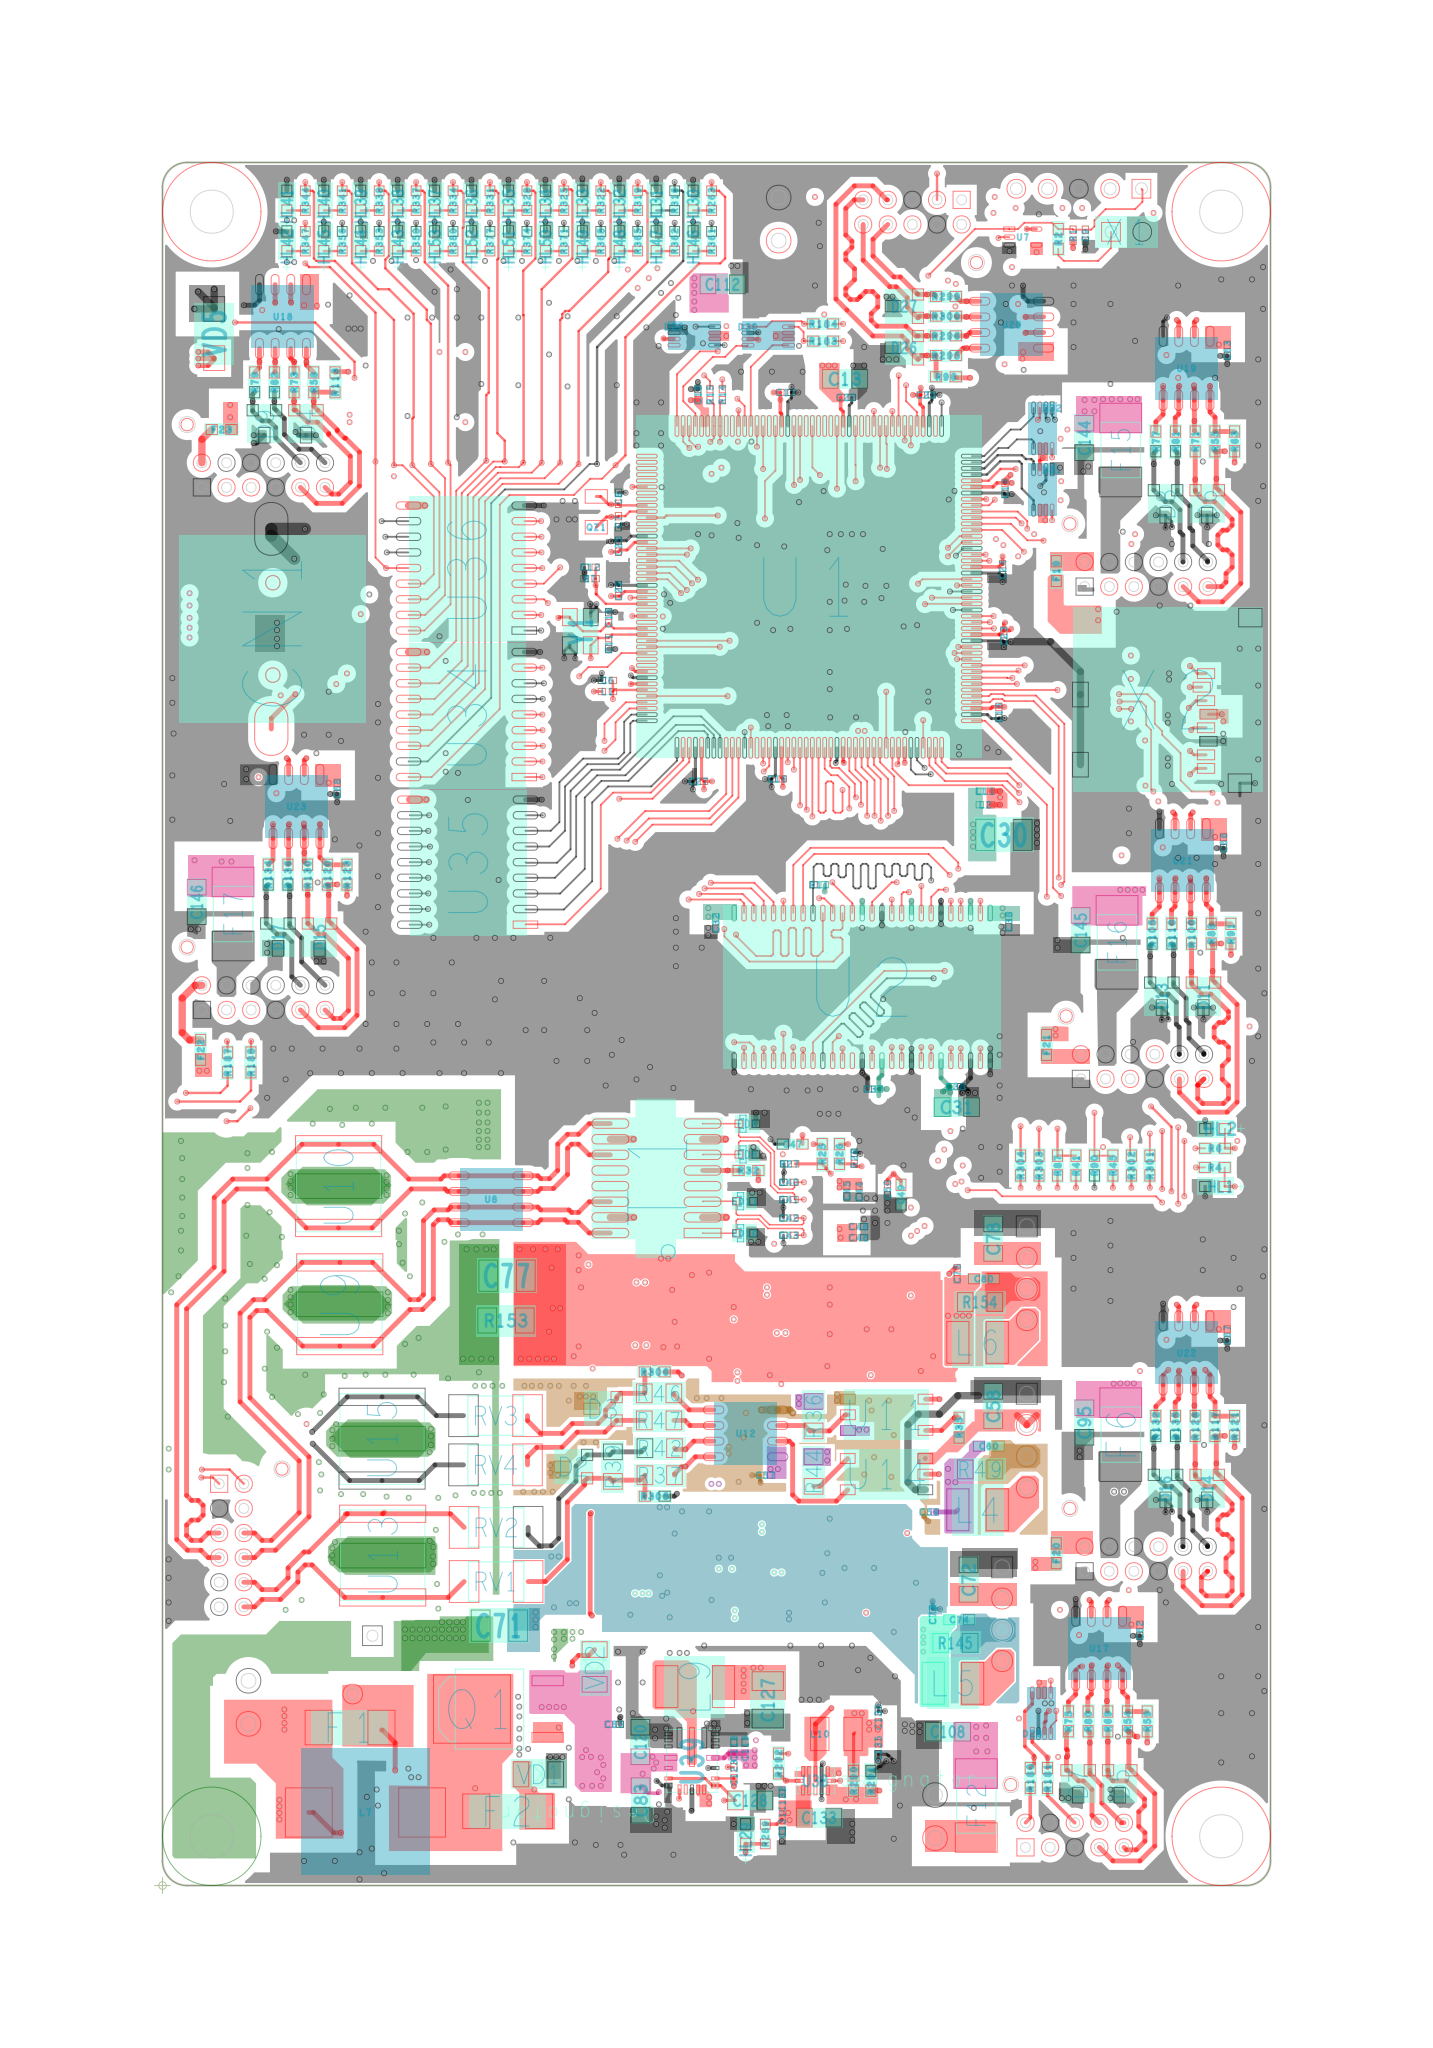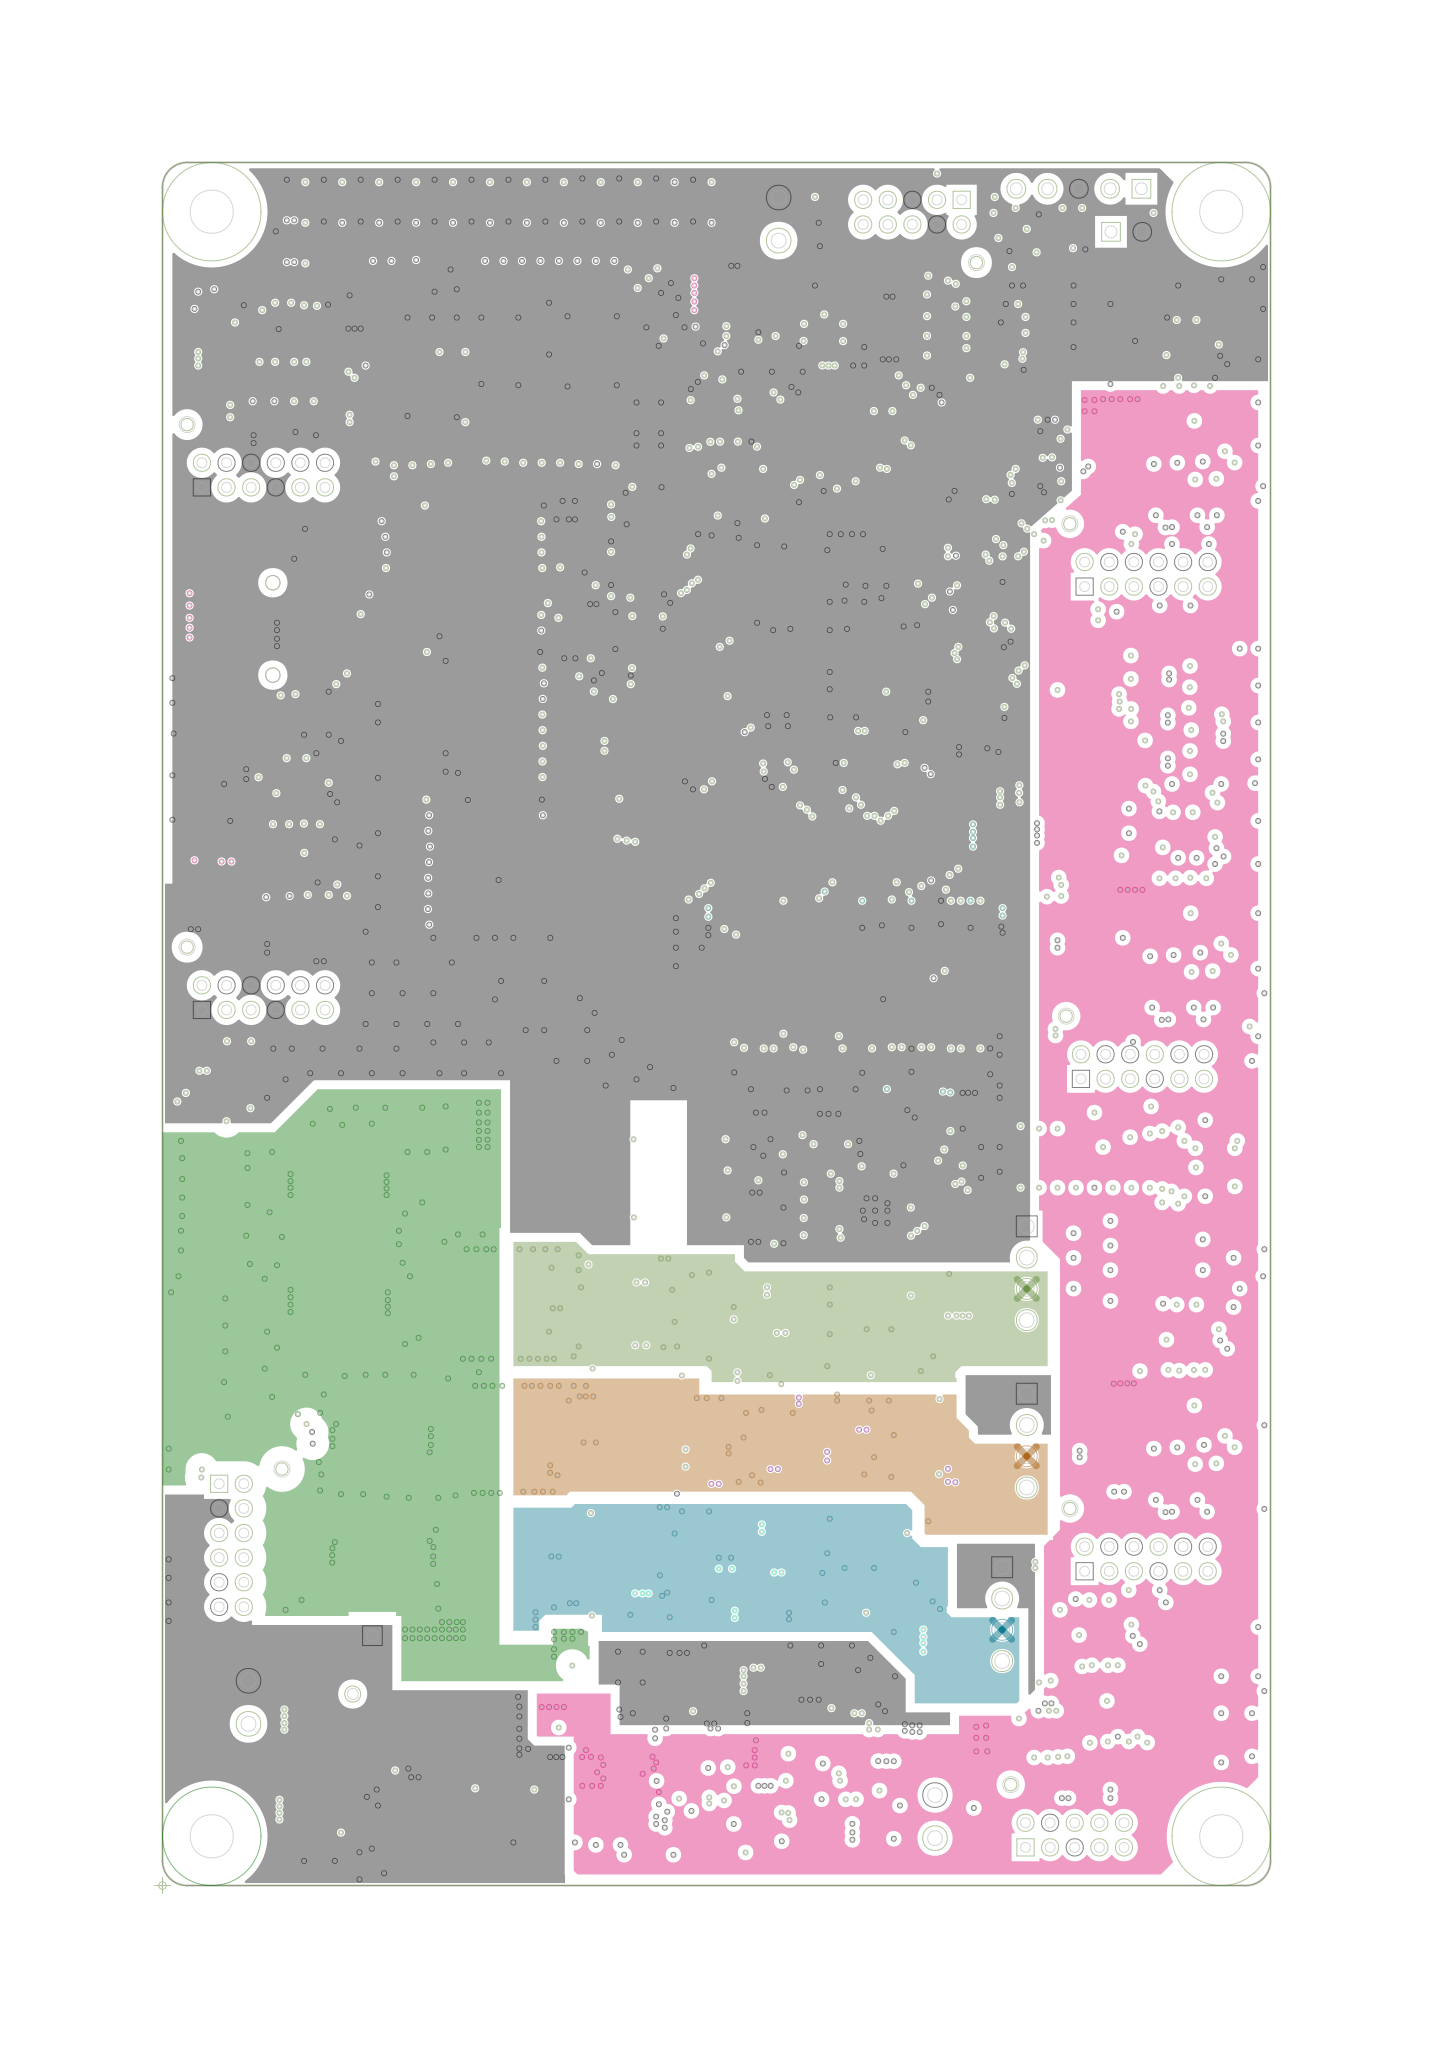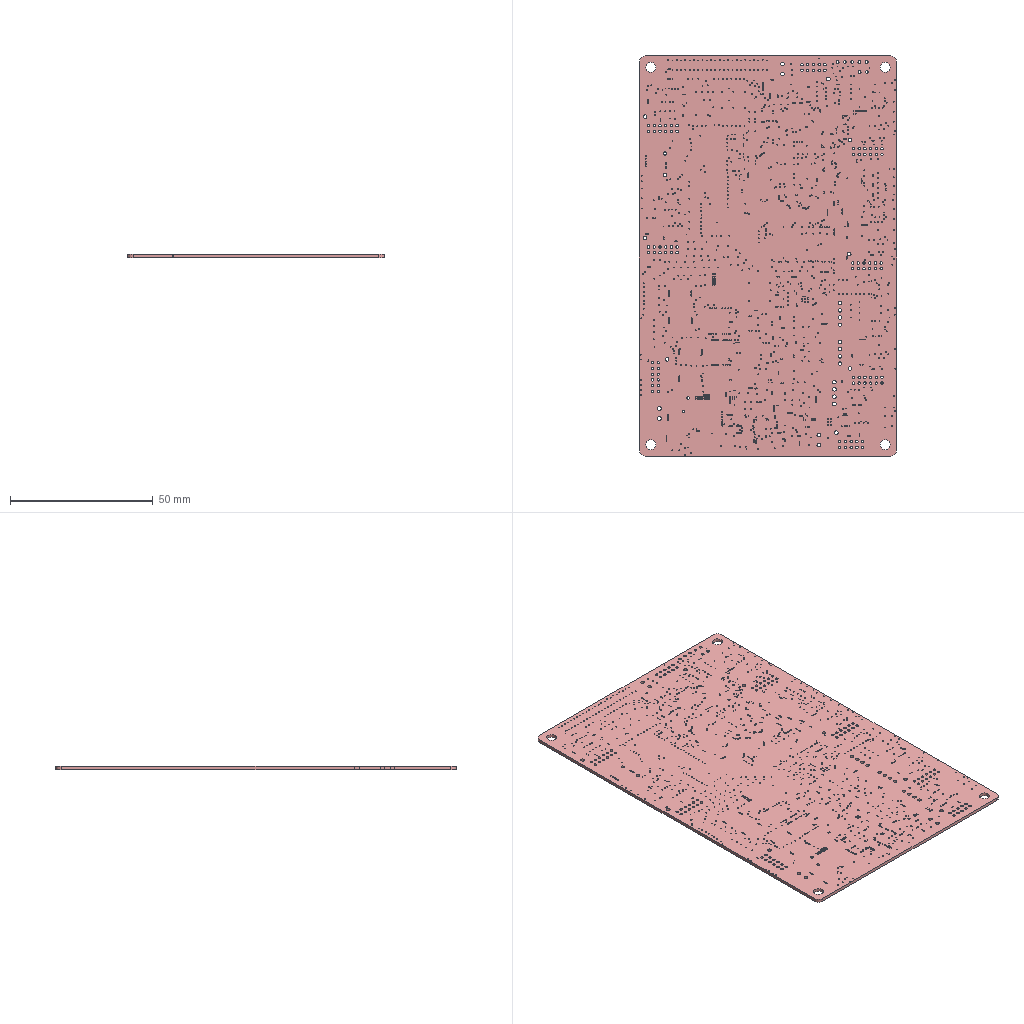Circuit board layout | Cadence Allegro | box 90 x 140 x 1.1 mm
Layer stack:
# Cadence Allegro layer stack of  (unit mm; from the constraint file cross-section; dielectric type: 0 not recorded (Allegro does not mark core vs prepreg), 3 surface material)
index,name,kind,layer,copper_thickness_mm,dielectric_type,dielectric_thickness_mm,dielectric_material,dielectric_constant
0,Top Surface,other,,,,,,
1,TOP,copper,TOP,0.0305,,,,
2,Dielectric1,dielectric,,,0,0.2032,FR-4,4.5
3,GND02,copper,GND02,0.0305,,,,
4,Dielectric2,dielectric,,,0,0.2032,FR-4,4.5
5,LAYER03,copper,LAYER03,0.0305,,,,
6,Dielectric3,dielectric,,,0,0.2032,FR-4,4.5
7,POWER04,copper,POWER04,0.0305,,,,
8,Dielectric4,dielectric,,,0,0.2032,FR-4,4.5
9,GND05,copper,GND05,0.0305,,,,
10,Dielectric5,dielectric,,,0,0.2032,FR-4,4.5
11,BOTTOM,copper,BOTTOM,0.0305,,,,
12,Bottom Surface,other,,,,,,
# drill layer pairs: low layer,high layer
drill_pair,TOP,BOTTOM
Part placement, first 524 of 796 lines:
REFDES,COMP_VALUE,SYM_NAME,SYM_X,SYM_Y,SYM_ROTATE,SYM_MIRROR
C1,2.2uf/16V,C0603,65.337,112.614,0.000,YES
C2,2.2uf/16V,C0603,59.537,92.914,270.000,YES
C3,1nf/50V,C0402,38.687,113.614,180.000,YES
C4,2.2uf/16V,C0603,37.237,97.914,270.000,YES
C5,0.1uf/50V,C0402,38.937,98.664,90.000,YES
C6,0.1uf/50V,C0402,36.587,97.914,180.000,NO
C7,6pf/50V,C0402,37.037,111.264,270.000,NO
C8,6pf/50V,C0402,37.037,112.264,90.000,NO
C9,0.1uf/50V,C0402,74.963,134.536,270.000,NO
C10,22pf/50V,C0402,36.237,102.564,90.000,NO
C11,22pf/50V,C0402,36.237,101.364,270.000,NO
C12,10nf/50V,C0402,35.187,107.114,180.000,NO
C13,4.7uf/50V,C0805,55.437,122.414,0.000,NO
C14,0.1uf/50V,C0402,55.487,90.514,0.000,YES
C15,0.1uf/50V,C0402,67.937,95.764,270.000,NO
C16,0.1uf/50V,C0402,50.387,89.914,180.000,NO
C17,0.1uf/50V,C0402,50.187,121.314,0.000,NO
C18,0.1uf/50V,C0402,43.486,120.687,90.000,NO
C19,0.1uf/50V,C0402,68.437,113.964,270.000,NO
C20,0.1uf/50V,C0402,60.737,91.964,270.000,YES
C21,4.7uf/50V,C0805,55.237,93.714,270.000,YES
C22,0.1uf/50V,C0402,55.087,120.914,0.000,NO
C23,0.1uf/50V,C0402,68.337,101.964,270.000,NO
C24,0.1uf/50V,C0402,68.237,107.364,270.000,NO
C25,0.1uf/50V,C0402,37.037,108.364,90.000,NO
C26,0.1uf/50V,C0402,37.037,104.764,90.000,NO
C27,0.1uf/50V,C0402,43.987,89.714,180.000,NO
C28,0.1uf/50V,C0402,61.587,121.114,0.000,NO
C29,10nf/50V,C0402,38.887,102.114,180.000,YES
C30,22uf/16V,C1210,68.349,85.363,0.000,NO
C31,4.7uf/50V,C0805,64.525,63.245,0.000,NO
C32,0.1uf/50V,C0402,44.937,78.664,270.000,NO
C33,0.1uf/50V,C0402,56.837,79.364,90.000,YES
C34,0.1uf/50V,C0402,60.837,79.364,90.000,YES
C35,0.1uf/50V,C0402,65.637,79.364,90.000,YES
C36,0.1uf/50V,C0402,68.737,78.764,270.000,NO
C37,0.1uf/50V,C0402,58.187,64.714,180.000,NO
C38,0.1uf/50V,C0402,63.987,64.914,0.000,NO
C39,0.1uf/50V,C0402,85.563,94.536,90.000,YES
C40,NC/10pF,C0402,51.336,57.137,180.000,NO
C41,NC/10pF,C0402,51.336,55.737,180.000,NO
C42,NC/10pF,C0402,51.336,54.237,180.000,NO
C43,NC/10pF,C0402,51.336,52.837,180.000,NO
C44,0.1uf/50V,C0402,56.586,56.837,270.000,NO
C45,0.1uf/50V,C0402,55.586,56.887,270.000,NO
C46,0.1uf/50V,C0402,56.086,52.637,0.000,NO
C47,10uf/16V,C0603,51.186,60.237,180.000,NO
C48,0.1uf/50V,C0402,56.086,53.537,0.000,NO
C49,10uf/16V,C0603,59.986,56.137,270.000,NO
C50,0.1uf/50V,C0402,58.886,56.987,270.000,NO
C51,0.1uf/50V,C0402,70.281,135.165,180.000,YES
C52,22pf/50V,C0402,58.136,59.037,0.000,YES
C53,22pf/50V,C0402,59.286,59.037,180.000,YES
C54,1NF/2KV,C1210,32.486,62.663,180.000,YES
C55,0.1uf/50V,C0402,44.936,60.663,0.000,YES
C56,0.1uf/50V,C0402,44.936,54.363,0.000,YES
C57,0.1uf/50V,C0402,49.436,33.337,180.000,NO
C58,4.7uf/50V,C0805,67.475,38.958,90.000,NO
C59,0.1uf/50V,C0402,62.736,30.352,180.000,NO
C60,10uf/16V,C0603,67.119,35.703,0.000,NO
C61,1NF/2KV,C1210,28.374,34.918,0.000,YES
C62,0.1uf/50V,C0402,79.386,21.187,270.000,NO
C63,0.1uf/50V,C0402,86.486,125.187,270.000,NO
C64,0.1uf/50V,C0402,12.550,129.200,180.000,YES
C65,0.1uf/50V,C0402,70.700,124.050,90.000,YES
C66,0.1uf/50V,C0402,86.186,85.187,270.000,NO
C67,0.1uf/50V,C0402,86.486,45.187,270.000,NO
C68,0.1uf/50V,C0402,14.186,89.587,270.000,NO
C69,0.1uf/50V,C0402,45.686,25.787,270.000,YES
C70,22pf/50V,C0402,34.186,21.887,270.000,YES
C71,1NF/2KV,C1210,27.363,21.114,180.000,NO
C72,4.7uf/50V,C0805,65.475,24.858,90.000,NO
C73,0.1uf/50V,C0402,62.552,21.564,90.000,NO
C74,10uf/16V,C0603,64.719,21.603,0.000,NO
C75,0.1uf/50V,C0402,64.552,49.264,90.000,NO
C76,22pf/50V,C0402,34.286,42.087,270.000,YES
C77,1NF/2KV,C1210,27.986,49.551,180.000,NO
C78,4.7uf/50V,C0805,67.475,52.558,90.000,NO
C79,0.1uf/50V,C0402,45.786,45.987,270.000,YES
C80,10uf/16V,C0603,66.719,49.303,0.000,NO
C83,10uf/50V,C0805,38.837,6.914,270.000,NO
C84,10uf/50V,C0805,38.763,6.614,90.000,YES
C85,0.1uf/50V,C0402,36.250,13.100,0.000,NO
C95,4.7uf/50V,C0805,74.879,37.619,270.000,NO
C96,0.1uf/50V,C0402,71.100,15.850,90.000,YES
C97,0.1uf/50V,C0402,71.850,12.500,0.000,YES
C102,0.1uf/50V,C0402,71.300,115.250,90.000,YES
C103,0.1uf/50V,C0402,71.300,111.650,270.000,YES
C105,0.1uf/50V,C0402,70.950,119.900,180.000,YES
C106,0.1uf/50V,C0402,71.300,116.650,270.000,YES
C108,4.7uf/50V,C0805,63.800,12.500,180.000,NO
C110,0.1uf/50V,C0402,45.050,125.900,0.000,YES
C111,0.1uf/50V,C0402,41.350,125.700,180.000,YES
C112,4.7uf/50V,C0805,45.500,130.100,0.000,NO
C113,0.1uf/50V,C0402,47.700,125.450,270.000,YES
C114,0.1uf/50V,C0402,50.450,125.900,180.000,YES
C115,10nf/50V,C0402,41.614,10.513,270.000,YES
C116,0.1uf/50V,C0402,40.714,10.513,270.000,YES
C117,0.1uf/50V,C0402,40.714,9.513,90.000,YES
C118,0.1uf/50V,C0402,46.414,10.713,90.000,NO
C119,10nf/50V,C0402,47.314,10.713,90.000,NO
C120,10uf/50V,C0805,38.814,11.663,90.000,NO
C121,10uf/50V,C0805,45.914,11.363,0.000,YES
C122,10uf/50V,C0805,38.714,11.263,270.000,YES
C123,0.47uf/25V,C0402,46.414,8.713,90.000,NO
C124,0.1uf/50V,C0402,43.850,6.600,0.000,YES
C125,22uf/16V,C1210,44.086,16.537,0.000,YES
C126,22uf/16V,C1210,49.137,15.086,90.000,YES
C127,22uf/16V,C1210,49.163,15.086,270.000,NO
C128,4.7uf/50V,C0805,47.737,6.914,0.000,NO
C129,0.1uf/50V,C0402,43.850,7.600,0.000,YES
C130,22uf/16V,C1210,53.437,4.814,180.000,YES
C131,10nf/50V,C0402,50.337,5.364,270.000,NO
C132,0.1uf/50V,C0402,50.337,6.564,90.000,NO
C133,10uf/50V,C0805,53.337,5.514,0.000,NO
C134,22pf/50V,C0402,56.137,7.764,270.000,YES
C135,0.1uf/50V,C0402,58.137,11.564,270.000,NO
C136,0.1uf/50V,C0402,58.137,13.264,90.000,NO
C137,22uf/16V,C1210,54.737,12.314,0.000,YES
C138,10nf/50V,C0402,54.350,8.500,0.000,YES
C139,0.1uf/50V,C0402,39.383,22.984,180.000,YES
C140,0.1uf/50V,C0402,39.483,43.184,180.000,YES
C141,1NF/2KV,C1210,33.586,17.437,270.000,YES
C142,10uf/50V,C0805,33.114,9.363,0.000,YES
C143,10uf/50V,C0805,35.763,12.686,270.000,YES
C144,4.7uf/50V,C0805,74.879,117.619,270.000,NO
C145,4.7uf/50V,C0805,74.579,77.619,270.000,NO
C146,4.7uf/50V,C0805,2.779,79.919,270.000,NO
C147,4.7uf/50V,C0805,6.981,101.021,180.000,YES
CN1,CR1220,CR1220,8.963,102.100,90.000,NO
D1,BAT54C,SOT23,13.163,99.472,0.000,YES
D2,SM712,SOT23,33.500,34.037,90.000,NO
D3,SM712,SOT23,35.900,38.737,90.000,NO
D4,SM712,SOT23,11.655,118.877,180.000,NO
D5,SM712,SOT23,77.755,8.377,180.000,NO
D6,SM712,SOT23,84.855,112.377,180.000,NO
D7,SM712,SOT23,74.376,8.377,180.000,NO
D8,SM712,SOT23,81.476,112.377,180.000,NO
D9,SM712,SOT23,8.276,118.877,180.000,NO
D11,SM712,SOT23,84.555,72.377,180.000,NO
D13,SM712,SOT23,81.176,72.377,180.000,NO
D14,SM712,SOT23,84.855,32.377,180.000,NO
D15,SM712,SOT23,12.755,77.177,180.000,NO
D16,SM712,SOT23,81.476,32.377,180.000,NO
D17,SM712,SOT23,9.376,77.177,180.000,NO
D18,SMC24,SOT23,33.100,25.937,90.000,YES
D19,TJA1044GT/3,SO8,43.926,28.142,0.000,YES
D20,SMC24,SOT23,33.000,46.137,90.000,YES
D21,TJA1044GT/3,SO8,44.026,48.342,0.000,YES
D26,SM712,SOT23,60.377,124.945,90.000,NO
D27,SM712,SOT23,60.377,128.324,90.000,NO
D28,TXS0102DCUR,VSSOP8,70.650,12.350,90.000,NO
D29,TXS0102DCUR,VSSOP8,41.551,126.659,0.000,NO
D30,TXS0102DCUR,VSSOP8,47.550,126.650,0.000,NO
D31,TXS0102DCUR,VSSOP8,72.259,115.049,270.000,NO
D32,TXS0102DCUR,VSSOP8,72.259,120.049,270.000,NO
ED8,ESD9X5VU,ESD5Z12T1,46.800,59.400,0.000,NO
ED9,ESD9X5VU,ESD5Z12T1,46.800,61.900,0.000,NO
ED10,ESD9X5VU,ESD5Z12T1,46.600,53.000,0.000,NO
ED11,ESD9X5VU,ESD5Z12T1,46.600,55.600,0.000,NO
F1,JFC2410-2100TS,JFC2410-2100TS,12.686,12.837,0.000,NO
F2,JFC2410-2100TS,JFC2410-2100TS,25.486,6.037,0.000,NO
F6,SMD1812P150TF/33,1812_2,77.837,36.634,90.000,NO
F12,SMD1812P150TF/33,1812_2,66.100,6.500,90.000,NO
F14,SMD1812P150TF/33,1812_2,47.400,129.400,0.000,YES
F15,SMD1812P150TF/33,1812_2,77.837,116.634,90.000,NO
F16,SMD1812P150TF/33,1812_2,77.537,76.634,90.000,NO
F17,SMD1812P150TF/33,1812_2,5.737,78.934,90.000,NO
F18,SMD1812P150TF/33,1812_2,4.737,107.066,90.000,YES
F19,0R,0603,72.600,106.800,270.000,NO
F20,0R,0603,72.600,27.000,270.000,NO
F21,0R,0603,71.800,68.300,90.000,NO
F22,0R,0603,3.100,67.900,270.000,NO
F23,0R,0603,4.800,118.300,0.000,NO
HL1,LED,LED0603,85.500,56.800,180.000,NO
HL2,LED,LED0603,85.500,61.500,180.000,NO
HL3,LED,LED0603,53.586,61.037,270.000,YES
HL4,LED,LED0603,54.986,61.037,270.000,YES
HL29,LED,LED0603,47.363,4.186,90.000,NO
HL30,LED,LED0603,43.100,136.900,90.000,NO
HL31,LED,LED0603,40.100,136.900,90.000,NO
HL32,LED,LED0603,37.100,136.900,90.000,NO
HL33,LED,LED0603,34.100,136.900,90.000,NO
HL34,LED,LED0603,31.100,136.900,90.000,NO
HL35,LED,LED0603,28.100,136.900,90.000,NO
HL36,LED,LED0603,25.100,136.900,90.000,NO
HL37,LED,LED0603,22.100,136.900,90.000,NO
HL38,LED,LED0603,19.100,136.900,90.000,NO
HL39,LED,LED0603,16.100,136.900,90.000,NO
HL40,LED,LED0603,13.100,136.900,90.000,NO
HL41,LED,LED0603,10.100,136.900,90.000,NO
HL42,LED,LED0603,10.100,133.600,90.000,NO
HL43,LED,LED0603,19.100,133.600,90.000,NO
HL44,LED,LED0603,16.100,133.600,90.000,NO
HL45,LED,LED0603,13.100,133.600,90.000,NO
HL46,LED,LED0603,43.100,133.600,90.000,NO
HL47,LED,LED0603,40.100,133.600,90.000,NO
HL48,LED,LED0603,37.100,133.600,90.000,NO
HL49,LED,LED0603,34.100,133.600,90.000,NO
HL50,LED,LED0603,31.100,133.600,90.000,NO
HL51,LED,LED0603,28.100,133.600,90.000,NO
HL52,LED,LED0603,25.100,133.600,90.000,NO
HL53,LED,LED0603,22.100,133.600,90.000,NO
HOLE1,HOLE,HOLEPAD_80X35,86.000,4.000,0.000,NO
HOLE2,HOLE,HOLEPAD_80X35,4.000,4.000,0.000,NO
HOLE3,HOLE,HOLEPAD_80X35,4.000,136.000,0.000,NO
HOLE4,HOLE,HOLEPAD_80X35,86.000,136.000,0.000,NO
J1,SIP5_2_1,SIP5,79.514,137.863,180.000,NO
L1,GZ1005D121TF,0402,35.687,97.014,0.000,NO
L2,GZ1005D601TF,0402,67.287,87.814,180.000,NO
L3,BLM18SG331TN1D,0603,51.186,60.237,0.000,YES
L4,WPN4020H1R0MT/5.8A,SM_IND_4,66.206,30.531,180.000,NO
L5,WPN4020H1R0MT/5.8A,SM_IND_4,64.206,16.431,180.000,NO
L6,WPN4020H1R0MT/5.8A,SM_IND_4,66.206,44.131,180.000,NO
L7,APS10A40M220,SM_IND_10X10,16.486,5.937,0.000,NO
L9,SMMS0530-2R2M/6.5A,SM_IND_5L,43.264,16.163,0.000,NO
L10,DFE252012PD-R47M=P2,SM_IND_3L,53.387,12.314,0.000,NO
L11,GZ1005D601TF,0402,67.287,88.914,180.000,NO
Q1,IRFR9024NTRPBF,TO252-2,27.286,14.337,180.000,NO
QZ1,XDMCZLNDDF-32.768KHZ,XTAL_SMD_3215,35.237,110.364,90.000,NO
R1,4.7K/1%,0402,73.963,133.636,90.000,NO
R2,100R/1%,0603,72.763,133.786,270.000,NO
R3,NC,0402,46.737,118.164,270.000,YES
R4,1K/1%,0603,85.475,58.344,0.000,NO
R5,100K/1%,0603,5.786,98.063,90.000,YES
R6,1K/1%,0603,85.500,59.900,0.000,NO
R7,10K/1%,0402,35.179,106.181,180.000,NO
R8,10K/1%,0402,47.837,119.064,90.000,YES
R9,10K/1%,0402,39.787,103.114,0.000,YES
R10,SDNT1608X103F3450FTF,0603,39.637,104.214,180.000,YES
R11,10K/1%,0402,53.787,81.314,180.000,NO
R12,0R,0402,45.401,116.716,90.000,YES
R13,0R,0402,44.374,116.719,90.000,YES
R14,NC,0402,45.472,120.686,90.000,NO
R15,NC,0402,44.472,120.683,90.000,NO
R16,10K/1%,0402,79.271,89.367,270.000,YES
R17,10K/1%,0402,79.263,93.036,90.000,YES
R18,10K/1%,0402,79.263,94.736,270.000,YES
R19,10K/1%,0402,79.263,98.036,90.000,YES
R20,10K/1%,0402,79.263,99.936,90.000,YES
R21,49.9R/1%,0603,50.486,57.137,180.000,YES
R22,49.9R/1%,0603,50.486,55.737,180.000,YES
R23,49.9R/1%,0603,50.486,54.237,180.000,YES
R24,49.9R/1%,0603,50.486,52.837,180.000,YES
R25,1k,0603,53.586,59.437,90.000,NO
R26,1k,0603,54.986,59.437,90.000,NO
R27,4.7K/1%,0402,51.386,58.637,180.000,NO
R28,4.7K/1%,0402,56.186,58.637,90.000,NO
R29,4.7K/1%,0402,68.150,135.200,180.000,YES
R30,12.1K/1%,0603,50.486,58.537,0.000,YES
R31,0R,0603,69.486,133.863,0.000,YES
R32,NC,0603,47.600,58.100,180.000,NO
R33,75/5%,1206,35.486,58.763,0.000,YES
R34,75/5%,1206,35.486,55.963,0.000,YES
R35,220R,0603,64.700,37.200,90.000,NO
R36,1K/1%,0805,52.886,38.137,270.000,NO
R37,10R/1%,0805,40.386,33.337,0.000,NO
R38,825R/1%,0603,43.986,34.037,0.000,YES
R39,120R/1%,0805,36.586,34.037,270.000,NO
R40,825R/1%,0603,43.986,35.437,0.000,YES
R41,100R,0603,74.200,58.500,270.000,NO
R42,10R/1%,0805,40.386,35.537,0.000,NO
R43,10K/1%,0402,77.200,58.450,90.000,YES
R44,330R,0805,52.886,33.637,270.000,NO
R45,100R,0603,77.200,58.500,270.000,NO
R46,10R/1%,0805,40.334,39.992,0.000,NO
R47,10R/1%,0805,40.337,37.792,0.000,NO
R48,1M,1206,28.414,38.105,0.000,YES
R49,220R,0805,66.406,33.810,180.000,NO
R50,10K/1%,0402,77.850,21.000,0.000,YES
R51,10K/1%,0402,74.450,21.000,180.000,YES
R52,10K/1%,0402,84.950,125.000,0.000,YES
R53,10K/1%,0402,81.550,125.000,180.000,YES
R54,10R/1%,0603,78.386,13.337,90.000,NO
R55,10R/1%,0603,85.486,117.337,90.000,NO
R56,10K/1%,0402,11.350,129.200,0.000,YES
R57,10K/1%,0402,8.250,129.200,180.000,YES
R58,10R/1%,0603,12.286,122.137,90.000,NO
R59,825R/1%,0603,79.986,13.337,90.000,NO
R60,100R/1%,0805,84.586,113.137,180.000,YES
R61,825R/1%,0603,76.786,13.337,270.000,YES
R62,100R/1%,0805,77.500,10.600,180.000,YES
R63,825R/1%,0603,87.086,117.337,90.000,NO
R64,825R/1%,0603,11.986,125.663,90.000,YES
R65,825R/1%,0603,10.414,125.663,90.000,YES
R66,100R/1%,0805,11.586,121.637,180.000,YES
R67,825R/1%,0603,83.886,117.337,270.000,YES
R68,0R,0603,77.686,22.337,0.000,YES
R69,10R/1%,0603,76.786,13.337,90.000,NO
R70,0R,0603,84.786,126.337,0.000,YES
R71,10R/1%,0603,83.886,117.337,90.000,NO
R72,0R,0603,11.700,130.500,0.000,YES
R73,10R/1%,0603,10.686,122.137,90.000,NO
R74,0R,0603,74.486,22.337,180.000,YES
R75,10R/1%,0603,73.586,13.337,90.000,NO
R76,0R,0603,81.586,126.337,180.000,YES
R77,10R/1%,0603,80.686,117.337,90.000,NO
R78,0R,0603,8.286,130.537,180.000,YES
R79,10R/1%,0603,7.486,122.137,90.000,NO
R80,10R/1%,0603,75.186,13.337,90.000,NO
R81,10R/1%,0603,82.286,117.337,90.000,NO
R82,10R/1%,0603,9.086,122.137,90.000,NO
R83,10K/1%,0402,70.700,125.250,270.000,YES
R84,10K/1%,0402,70.700,128.350,90.000,YES
R85,10K/1%,0402,84.650,85.000,0.000,YES
R86,10K/1%,0402,81.250,85.000,180.000,YES
R87,NC,0603,72.700,58.500,270.000,NO
R88,10R/1%,0603,85.186,77.337,90.000,NO
R90,NC,0603,75.700,58.500,270.000,NO
R91,825R/1%,0603,86.786,77.337,90.000,NO
R92,825R/1%,0603,83.586,77.337,270.000,YES
R93,100R/1%,0805,84.286,73.137,180.000,YES
R94,NC,0603,79.986,13.337,90.000,YES
R95,NC,0603,73.586,13.337,90.000,YES
R96,NC,0603,63.637,122.586,180.000,NO
R97,NC,0603,63.637,129.114,0.000,YES
R98,0R,0603,72.037,125.314,270.000,YES
R99,0R,0603,84.486,86.337,0.000,YES
R100,10R/1%,0603,83.586,77.337,90.000,NO
R101,NC,0603,87.086,37.337,90.000,YES
R102,NC,0603,80.686,37.337,90.000,YES
R103,0R,0603,72.037,128.314,90.000,YES
R104,0R,0603,81.286,86.337,180.000,YES
R105,10R/1%,0603,80.386,77.337,90.000,NO
R106,NC,0603,87.086,117.337,90.000,YES
R107,NC,0603,80.686,117.337,90.000,YES
R108,NC,0603,86.786,77.337,90.000,YES
R109,NC,0603,80.386,77.337,90.000,YES
R110,10R/1%,0603,81.986,77.337,90.000,NO
R111,NC,0603,14.986,82.137,90.000,YES
R112,NC,0603,8.586,82.137,90.000,YES
R113,NC,0603,14.014,122.137,270.000,NO
R114,NC,0603,7.486,122.137,90.000,YES
R115,10K/1%,0402,84.950,45.000,0.000,YES
R116,10K/1%,0402,81.550,45.000,180.000,YES
R117,10R/1%,0603,85.486,37.337,90.000,NO
R118,10K/1%,0402,12.650,89.400,0.000,YES
R119,10K/1%,0402,9.250,89.400,180.000,YES
R120,10R/1%,0603,13.386,82.137,90.000,NO
R121,825R/1%,0603,87.086,37.337,90.000,NO
R122,100R/1%,0805,84.586,33.137,180.000,YES
R123,825R/1%,0603,14.986,82.137,90.000,NO
R124,100R/1%,0805,12.600,79.400,180.000,YES
R125,825R/1%,0603,83.886,37.337,270.000,YES
R126,825R/1%,0603,11.786,82.137,270.000,YES
R127,0R,0603,84.786,46.337,0.000,YES
R128,10R/1%,0603,83.886,37.337,90.000,NO
R129,0R,0603,12.486,90.737,0.000,YES
R130,10R/1%,0603,11.786,82.137,90.000,NO
R131,0R,0603,81.586,46.337,180.000,YES
R132,10R/1%,0603,80.686,37.337,90.000,NO
R133,0R,0603,9.286,90.737,180.000,YES
R134,10R/1%,0603,8.586,82.137,90.000,NO
R135,10R/1%,0603,82.286,37.337,90.000,NO
R136,10R/1%,0603,10.186,82.137,90.000,NO
R137,220R,0603,59.086,24.637,0.000,YES
R138,1K/1%,0805,47.686,23.237,270.000,YES
R139,1K/1%,0603,39.586,29.637,0.000,YES
R140,1K/1%,0603,58.386,27.837,270.000,YES
R141,499R,0805,47.686,27.837,90.000,YES
R142,62R/1%,1206,36.186,23.437,270.000,YES
R143,62R/1%,1206,36.186,28.737,90.000,YES
R144,1M,1206,27.400,21.400,0.000,YES
R145,220R,0805,64.406,19.710,180.000,NO
R146,220R,0603,59.386,43.937,0.000,YES
R147,1K/1%,0805,47.986,42.537,270.000,YES
R148,1K/1%,0603,40.000,50.200,0.000,YES
R149,1K/1%,0603,58.686,47.137,270.000,YES
R150,499R,0805,47.986,47.137,90.000,YES
R151,62R/1%,1206,36.286,43.637,270.000,YES
R152,62R/1%,1206,36.286,48.937,90.000,YES
R153,1M,1206,27.901,45.909,180.000,NO
R154,220R,0805,66.406,47.410,180.000,NO
R173,10K/1%,0402,71.850,11.000,180.000,YES
R174,10K/1%,0402,70.450,11.000,0.000,YES
R176,10K/1%,0402,72.300,115.150,90.000,YES
R177,10K/1%,0402,72.300,111.650,270.000,YES
R178,10K/1%,0402,73.250,119.100,180.000,YES
R179,10K/1%,0402,72.300,116.650,270.000,YES
R180,100R/1%,0603,70.486,8.737,90.000,NO
R181,100R/1%,0603,71.886,8.737,90.000,NO
R182,10K/1%,0402,44.150,126.900,180.000,YES
R183,100R/1%,0603,53.663,125.486,180.000,NO
R184,100R/1%,0603,53.663,126.886,180.000,NO
R185,10K/1%,0402,52.850,126.900,180.000,YES
R186,10K/1%,0402,52.850,125.500,180.000,YES
R187,NC,0603,5.289,66.881,90.000,NO
R188,NC,0603,7.186,66.881,90.000,NO
R189,0R,0603,5.238,66.881,270.000,YES
R190,0R,0603,7.141,66.881,270.000,YES
R191,1K/1%,R0603,36.800,117.300,270.000,YES
R194,1K/1%,R0603,33.800,117.300,270.000,YES
R195,1K/1%,R0603,43.100,136.900,270.000,YES
R196,1K/1%,R0603,44.600,136.900,270.000,YES
R209,1K/1%,R0603,35.300,117.300,270.000,YES
R210,1K/1%,R0603,32.300,117.300,270.000,YES
R211,1K/1%,R0603,30.800,117.300,270.000,YES
R212,1K/1%,R0603,29.300,117.300,270.000,YES
R213,1K/1%,R0603,27.800,117.300,270.000,YES
R214,1K/1%,R0603,26.300,117.300,270.000,YES
R215,1K/1%,R0603,23.300,117.300,270.000,YES
R216,1K/1%,R0603,21.800,117.300,270.000,YES
R217,1K/1%,R0603,20.300,117.300,270.000,YES
R218,1K/1%,R0603,18.800,117.300,270.000,YES
R219,1K/1%,R0603,17.300,117.300,270.000,YES
R220,1K/1%,R0603,20.600,130.500,270.000,YES
R221,1K/1%,R0603,18.600,130.500,270.000,YES
R222,1K/1%,R0603,17.100,130.500,270.000,YES
R239,1K/1%,R0603,36.700,130.500,270.000,YES
R240,1K/1%,R0603,35.200,130.500,270.000,YES
R241,1K/1%,R0603,33.700,130.500,270.000,YES
R242,1K/1%,R0603,32.200,130.500,270.000,YES
R243,1K/1%,R0603,30.700,130.500,270.000,YES
R244,1K/1%,R0603,29.200,130.500,270.000,YES
R245,1K/1%,R0603,27.700,130.500,270.000,YES
R246,1K/1%,R0603,26.200,130.500,270.000,YES
R263,1K/1%,R0603,44.600,136.900,270.000,NO
R287,10K/1%,0402,40.950,7.600,180.000,YES
R288,4.7K/1%,0402,40.950,6.600,180.000,YES
R289,1K/1%,R0603,48.963,4.186,270.000,NO
R290,88.7K/1%,0603,56.137,8.514,270.000,NO
R291,19.6K/1%,0603,57.537,8.514,270.000,NO
R292,10K/1%,0603,50.037,9.914,90.000,NO
R293,8.06K/1%,0402,53.387,9.414,180.000,YES
R294,100R/1%,0805,63.137,125.014,90.000,YES
R295,10R/1%,0603,63.637,124.314,0.000,NO
R296,10R/1%,0603,63.637,125.914,0.000,NO
R297,825R/1%,0603,67.163,124.614,0.000,YES
R298,825R/1%,0603,67.163,126.186,0.000,YES
R299,10R/1%,0603,63.637,129.114,0.000,NO
R300,10R/1%,0603,63.637,127.514,0.000,NO
R301,100R,0603,80.200,58.500,270.000,NO
R302,100R,0603,78.700,58.500,270.000,NO
R303,100R,0603,71.200,58.500,270.000,NO
R304,100R,0603,69.700,58.500,270.000,NO
R305,NC,0603,39.986,31.634,180.000,NO
R306,NC,0603,39.983,41.734,180.000,NO
R307,1M,1206,30.300,17.200,270.000,YES
R309,10K/1%,0603,32.986,13.737,180.000,YES
R310,47K/1%,0603,32.986,12.037,0.000,YES
R316,1K/1%,R0603,41.600,136.900,270.000,NO
R317,1K/1%,R0603,41.600,136.900,270.000,YES
R318,1K/1%,R0603,40.100,136.900,270.000,YES
R319,1K/1%,R0603,38.600,136.900,270.000,NO
R320,1K/1%,R0603,37.100,136.900,270.000,YES
R321,1K/1%,R0603,38.600,136.900,270.000,YES
R322,1K/1%,R0603,35.600,136.900,270.000,NO
R323,1K/1%,R0603,34.100,136.900,270.000,YES
R324,1K/1%,R0603,35.600,136.900,270.000,YES
R325,1K/1%,R0603,32.600,136.900,270.000,NO
R326,1K/1%,R0603,32.600,136.900,270.000,YES
R327,1K/1%,R0603,31.100,136.900,270.000,YES
R328,1K/1%,R0603,29.600,136.900,270.000,NO
R329,1K/1%,R0603,28.100,136.900,270.000,YES
R330,1K/1%,R0603,29.600,136.900,270.000,YES
R331,1K/1%,R0603,26.600,136.900,270.000,NO
R332,1K/1%,R0603,25.100,136.900,270.000,YES
R333,1K/1%,R0603,26.600,136.900,270.000,YES
R334,1K/1%,R0603,23.600,136.900,270.000,NO
R335,1K/1%,R0603,23.600,136.900,270.000,YES
R336,1K/1%,R0603,22.100,136.900,270.000,YES
R337,1K/1%,R0603,20.600,136.900,270.000,NO
R338,1K/1%,R0603,17.600,136.900,270.000,NO
R339,1K/1%,R0603,17.600,136.900,270.000,YES
R340,1K/1%,R0603,16.100,136.900,270.000,YES
R341,1K/1%,R0603,14.600,136.900,270.000,NO
R342,1K/1%,R0603,13.100,136.900,270.000,YES
R343,1K/1%,R0603,14.600,136.900,270.000,YES
R344,1K/1%,R0603,11.600,136.900,270.000,NO
R345,1K/1%,R0603,10.100,136.900,270.000,YES
R346,1K/1%,R0603,11.600,136.900,270.000,YES
R347,1K/1%,R0603,11.600,133.600,270.000,NO
R348,1K/1%,R0603,11.600,133.600,270.000,YES
R349,1K/1%,R0603,10.100,133.600,270.000,YES
R350,1K/1%,R0603,20.600,133.600,270.000,NO
R351,1K/1%,R0603,20.600,133.600,270.000,YES
R352,1K/1%,R0603,19.100,133.600,270.000,YES
R353,1K/1%,R0603,17.600,133.600,270.000,NO
R354,1K/1%,R0603,16.100,133.600,270.000,YES
R355,1K/1%,R0603,17.600,133.600,270.000,YES
R356,1K/1%,R0603,14.600,133.600,270.000,NO
R357,1K/1%,R0603,13.100,133.600,270.000,YES
R358,1K/1%,R0603,14.600,133.600,270.000,YES
R359,1K/1%,R0603,19.100,136.900,270.000,YES
R360,1K/1%,R0603,20.600,136.900,270.000,YES
R361,1K/1%,R0603,44.600,133.600,270.000,NO
R362,1K/1%,R0603,41.600,133.600,270.000,NO
R363,1K/1%,R0603,40.100,133.600,270.000,YES
R364,1K/1%,R0603,41.600,133.600,270.000,YES
R365,1K/1%,R0603,38.600,133.600,270.000,NO
R366,1K/1%,R0603,38.600,133.600,270.000,YES
R367,1K/1%,R0603,37.100,133.600,270.000,YES
R368,1K/1%,R0603,35.600,133.600,270.000,NO
R369,1K/1%,R0603,35.600,133.600,270.000,YES
R370,1K/1%,R0603,34.100,133.600,270.000,YES
R371,1K/1%,R0603,32.600,133.600,270.000,NO
R372,1K/1%,R0603,32.600,133.600,270.000,YES
R373,1K/1%,R0603,31.100,133.600,270.000,YES
R374,1K/1%,R0603,29.600,133.600,270.000,NO
R375,1K/1%,R0603,29.600,133.600,270.000,YES
R376,1K/1%,R0603,28.100,133.600,270.000,YES
R377,1K/1%,R0603,26.600,133.600,270.000,NO
R378,1K/1%,R0603,26.600,133.600,270.000,YES
R379,1K/1%,R0603,25.100,133.600,270.000,YES
R380,1K/1%,R0603,23.600,133.600,270.000,NO
R381,1K/1%,R0603,22.100,133.600,270.000,YES
R382,1K/1%,R0603,23.600,133.600,270.000,YES
R383,1K/1%,R0603,44.600,133.600,270.000,YES
R384,1K/1%,R0603,43.100,133.600,270.000,YES
RV1,SMD1812P050TF,1812_2,27.100,24.700,180.000,NO
RV2,SMD1812P050TF,1812_2,27.100,29.100,180.000,NO
RV3,SMD1812P050TF,1812_2,27.051,38.180,180.000,NO
RV4,SMD1812P050TF,1812_2,27.048,34.180,180.000,NO
RV5,SMD1812P050TF,1812_2,27.100,24.700,0.000,YES
RV6,SMD1812P050TF,1812_2,27.100,29.100,0.000,YES
RV7,SMD1812P050TF,1812_2,26.586,45.237,0.000,YES
RV8,SMD1812P050TF,1812_2,26.486,49.237,0.000,YES
RV9,820KD07J,10D151K,17.050,20.300,90.000,YES
T1,HX1188NL,TRANS_H1102,43.869,53.018,180.000,NO
TP1,TESTPOINT,TESTPOINT-33MIL,59.037,12.414,270.000,YES
TP2,TESTPOINT,TESTPOINT-33MIL,84.700,58.400,0.000,YES
TP3,TESTPOINT,TESTPOINT-33MIL,84.700,60.200,0.000,YES
TP4,TESTPOINT,TESTPOINT-33MIL,87.800,56.800,0.000,YES
Pad and via stacks:
# Allegro (Cadence) via spans and padstacks; design units: ("millimeters" 3 1000)
# via spans: padstack,start_layer,end_layer,net_example,count
# Allegro padstack definitions: name,start_layer,end_layer,drill,plating,holeType,type
SR36X32,"ETCH/TOP","ETCH/TOP",0.0,"PLATED","none","smd"
SR2500X2400M,"ETCH/TOP","ETCH/TOP",0.0,"PLATED","none","smd"
SR36X36,"ETCH/TOP","ETCH/TOP",0.0,"PLATED","none","smd"
SR1000X800M,"ETCH/TOP","ETCH/TOP",0.0,"PLATED","none","smd"
SR1500X600M,"ETCH/TOP","ETCH/TOP",0.0,"PLATED","none","smd"
SR2700X1500M,"ETCH/TOP","ETCH/TOP",0.0,"PLATED","none","smd"
SR60X100,"ETCH/TOP","ETCH/TOP",0.0,"PLATED","none","smd"
CO60X35,"ETCH/TOP","ETCH/BOTTOM",3.5,"PLATED","circle_drill","through"
TS1000X600M,"ETCH/TOP","ETCH/BOTTOM",0.6,"PLATED","circle_drill","through"
TC1000X600M,"ETCH/TOP","ETCH/BOTTOM",0.6,"PLATED","circle_drill","through"
CO50X30,"ETCH/TOP","ETCH/BOTTOM",3.0,"PLATED","circle_drill","through"
VIA22D12,"ETCH/TOP","ETCH/BOTTOM",0.305,"PLATED","circle_drill","through"
VIA20D10,"ETCH/TOP","ETCH/BOTTOM",0.254,"PLATED","circle_drill","through"
SMDS0R8X0R8MM,"ETCH/TOP","ETCH/TOP",0.0,"NON_PLATED","none","smd"
SMD0R46X0R5MM,"ETCH/TOP","ETCH/TOP",0.0,"NON_PLATED","none","smd"
SR60X50,"ETCH/TOP","ETCH/TOP",0.0,"PLATED","none","smd"
NPAD46,"ETCH/TOP","ETCH/BOTTOM",1.168,"NON_PLATED","circle_drill","through"
SMD4R3X2R7MMOB,"ETCH/TOP","ETCH/TOP",0.0,"NON_PLATED","none","smd"
SMD0R91X0R91MM,"ETCH/TOP","ETCH/TOP",0.0,"NON_PLATED","none","smd"
SMD0R9X1R27MM,"ETCH/TOP","ETCH/TOP",0.0,"NON_PLATED","none","smd"
SO80X20,"ETCH/TOP","ETCH/TOP",0.0,"PLATED","none","smd"
SO1000X300M,"ETCH/TOP","ETCH/TOP",0.0,"PLATED","none","smd"
SR1000X300M,"ETCH/TOP","ETCH/TOP",0.0,"PLATED","none","smd"
SMD0R93X0R98MM,"ETCH/TOP","ETCH/TOP",0.0,"NON_PLATED","none","smd"
TR38X60,"ETCH/TOP","ETCH/BOTTOM",0.965,"PLATED","circle_drill","through"
TC38X60,"ETCH/TOP","ETCH/BOTTOM",0.965,"PLATED","circle_drill","through"
SR600X500M,"ETCH/TOP","ETCH/TOP",0.0,"PLATED","none","smd"
SR3400X1800M,"ETCH/TOP","ETCH/TOP",0.0,"PLATED","none","smd"
SR4000X3800M,"ETCH/TOP","ETCH/TOP",0.0,"PLATED","none","smd"
SMD0R8X0R8MM,"ETCH/TOP","ETCH/TOP",0.0,"NON_PLATED","none","smd"
SR60X80,"ETCH/TOP","ETCH/TOP",0.0,"PLATED","none","smd"
SR3400X2400M,"ETCH/TOP","ETCH/TOP",0.0,"PLATED","none","smd"
TS1600X900M,"ETCH/TOP","ETCH/BOTTOM",0.9,"PLATED","circle_drill","through"
TO1600X900M,"ETCH/TOP","ETCH/BOTTOM",0.9,"PLATED","circle_drill","through"
SR3000X760M,"ETCH/TOP","ETCH/TOP",0.0,"PLATED","none","smd"
SO3000X760M,"ETCH/TOP","ETCH/TOP",0.0,"PLATED","none","smd"
SMD0R3X1R7OBMM,"ETCH/TOP","ETCH/TOP",0.0,"NON_PLATED","none","smd"
TC1300X2300M,"ETCH/TOP","ETCH/BOTTOM",1.3,"PLATED","circle_drill","through"
SR1200X800M,"ETCH/TOP","ETCH/TOP",0.0,"PLATED","none","smd"
SMD1R65X0R64MM,"ETCH/TOP","ETCH/TOP",0.0,"NON_PLATED","none","smd"
TS1700X1200M,"ETCH/TOP","ETCH/BOTTOM",1.2,"PLATED","circle_drill","through"
TC1700X1200M,"ETCH/TOP","ETCH/BOTTOM",1.2,"PLATED","circle_drill","through"
SMD1R3X0R35MM,"ETCH/TOP","ETCH/TOP",0.0,"NON_PLATED","none","smd"
SR8000X2400M,"ETCH/TOP","ETCH/TOP",0.0,"PLATED","none","smd"
SR2000X600M,"ETCH/TOP","ETCH/TOP",0.0,"PLATED","none","smd"
SO2000X600M,"ETCH/TOP","ETCH/TOP",0.0,"PLATED","none","smd"
SMD1X0R3MM,"ETCH/TOP","ETCH/TOP",0.0,"NON_PLATED","none","smd"
SMD0R3X1MM,"ETCH/TOP","ETCH/TOP",0.0,"NON_PLATED","none","smd"
SMD2R5X2R5MM,"ETCH/TOP","ETCH/TOP",0.0,"NON_PLATED","none","smd"
SR900X350M,"ETCH/TOP","ETCH/TOP",0.0,"PLATED","none","smd"
SO900X350M,"ETCH/TOP","ETCH/TOP",0.0,"PLATED","none","smd"
SR50X80,"ETCH/TOP","ETCH/TOP",0.0,"PLATED","none","smd"
SR2000X1700M,"ETCH/TOP","ETCH/TOP",0.0,"PLATED","none","smd"
TC1200X2000M,"ETCH/TOP","ETCH/BOTTOM",1.2,"PLATED","circle_drill","through"
TS1400X800M,"ETCH/TOP","ETCH/BOTTOM",0.8,"PLATED","circle_drill","through"
TC1400X800M,"ETCH/TOP","ETCH/BOTTOM",0.8,"PLATED","circle_drill","through"
HOLE1300M,"ETCH/TOP","ETCH/BOTTOM",1.3,"NON_PLATED","circle_drill","through"
SR1600X700M,"ETCH/TOP","ETCH/TOP",0.0,"PLATED","none","smd"
HOLE1000M,"ETCH/TOP","ETCH/BOTTOM",1.0,"PLATED","circle_drill","through"
SR1500X1200M,"ETCH/TOP","ETCH/TOP",0.0,"PLATED","none","smd"
SR2200X1200M,"ETCH/TOP","ETCH/TOP",0.0,"PLATED","none","smd"
SR1600X1500M,"ETCH/TOP","ETCH/TOP",0.0,"PLATED","none","smd"
SR1400X1200M,"ETCH/TOP","ETCH/TOP",0.0,"PLATED","none","smd"
R10160240000000A,"ETCH/TOP","ETCH/TOP",0.0,"NON_PLATED","none","smd"
R10100240000000A,"ETCH/TOP","ETCH/TOP",0.0,"NON_PLATED","none","smd"
R10160390000007A,"ETCH/TOP","ETCH/TOP",0.0,"NON_PLATED","none","smd"
R10160650000007A,"ETCH/TOP","ETCH/TOP",0.0,"NON_PLATED","none","smd"
R10161240000007A,"ETCH/TOP","ETCH/TOP",0.0,"NON_PLATED","none","smd"
R10100300000000A,"ETCH/TOP","ETCH/TOP",0.0,"NON_PLATED","none","smd"
SR2800X2200,"ETCH/TOP","ETCH/TOP",0.0,"PLATED","none","smd"
SR1800X1100M,"ETCH/TOP","ETCH/TOP",0.0,"PLATED","none","smd"
V10160160080000A,"ETCH/TOP","ETCH/BOTTOM",0.203,"PLATED","circle_drill","through"
R10310100000215A,"ETCH/TOP","ETCH/TOP",0.0,"NON_PLATED","none","smd"
R10910100000245A,"ETCH/TOP","ETCH/TOP",0.0,"NON_PLATED","none","smd"
R10260100000200A,"ETCH/TOP","ETCH/TOP",0.0,"NON_PLATED","none","smd"
SR1400X800M,"ETCH/TOP","ETCH/TOP",0.0,"PLATED","none","smd"
SR1900X1500M,"ETCH/TOP","ETCH/TOP",0.0,"PLATED","none","smd"
SR2000X1280M,"ETCH/TOP","ETCH/TOP",0.0,"PLATED","none","smd"
T_33MIL,"ETCH/TOP","ETCH/TOP",0.0,"PLATED","none","smd"
SR7000X1400M,"ETCH/TOP","ETCH/TOP",0.0,"PLATED","none","smd"
SR7000X2000M,"ETCH/TOP","ETCH/TOP",0.0,"PLATED","none","smd"
VIA10X16MIL,"ETCH/TOP","ETCH/BOTTOM",0.254,"PLATED","circle_drill","through"
VIA300X500MNS,"ETCH/TOP","ETCH/BOTTOM",0.3,"PLATED","circle_drill","through"
SMD2R65X0R8MM,"ETCH/TOP","ETCH/TOP",0.0,"NON_PLATED","none","smd"
SMD6R25X5R55MM,"ETCH/TOP","ETCH/TOP",0.0,"NON_PLATED","none","smd"
SS600M,"ETCH/TOP","ETCH/TOP",0.0,"PLATED","none","smd"
SS300M,"ETCH/TOP","ETCH/TOP",0.0,"PLATED","none","smd"
SR1600X600M,"ETCH/TOP","ETCH/TOP",0.0,"PLATED","none","smd"
SR1800X1750M,"ETCH/TOP","ETCH/TOP",0.0,"PLATED","none","smd"
CO80X35,"ETCH/TOP","ETCH/BOTTOM",3.5,"PLATED","circle_drill","through"
Design rules, without the lines most boards share, first 7 of 45 lines:
# Cadence Allegro design rules of  (from the Constraint Manager export constraints.dcfx, design unit mm; typed fields in mm)
# columns: name | kind | enabled | priority | scope1 | scope2 | descriptor | typed fields (field=value)
# Allegro precedence (priority 1 wins): 1 Region class-to-class, 2 Region class, 3 Region, 4 class-to-class, 5 DiffPair/Bus/NetGroup override, 6 NetClass, 7 constraint set (CSet) default
# per-layer values are written LAYER=value in the descriptor and LAYER:mm in the typed field; a maximum of 0 means no limit set
# --- net classes (and buses / net groups) ---
# (no net classes defined: every net uses the default constraint sets)
# --- track widths, neck and differential-pair gap (physical constraint sets) ---